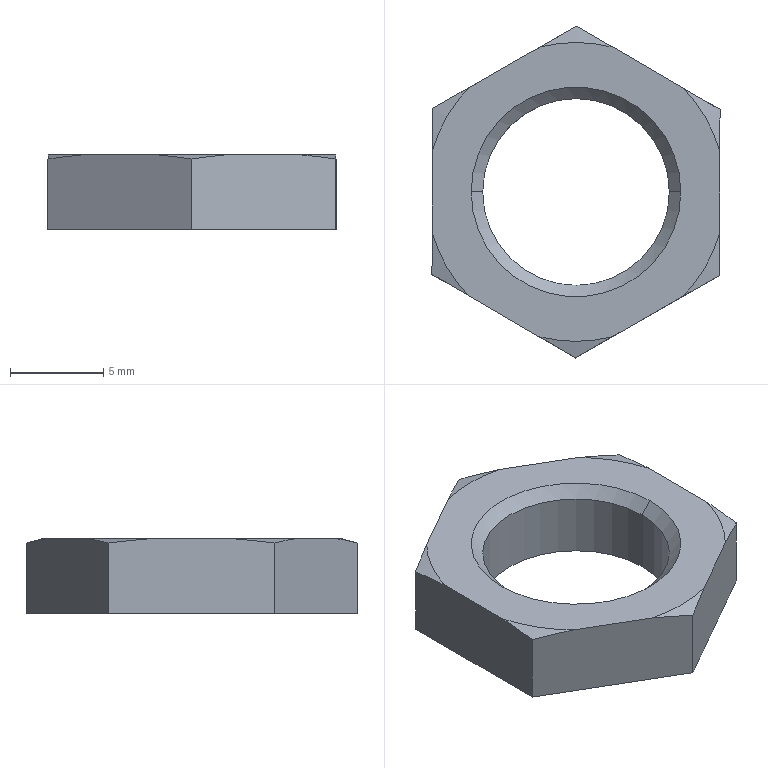Part | SolidWorks | features Cut 3, Chamfer 1, Extrusion 1 | 1 solid | 18 faces | box 15.424 x 17.77 x 4 mm | volume 499.386 mm3 | cone 8 | plane 8 | cylinder 2 | commonest cylinder face diameters 10 x2
STEP:
#1=CARTESIAN_POINT('',(-5.,0.,7.787));
#2=VERTEX_POINT('',#1);
#3=CARTESIAN_POINT('',(5.,0.,7.787));
#4=VERTEX_POINT('',#3);
#5=CARTESIAN_POINT('',(0.,0.,7.787));
#6=DIRECTION('',(0.,0.,1.));
#7=DIRECTION('',(-1.,0.,0.));
#8=AXIS2_PLACEMENT_3D('',#5,#6,#7);
#9=CIRCLE('',#8,5.);
#10=EDGE_CURVE('',#2,#4,#9,.T.);
#11=ORIENTED_EDGE('',*,*,#10,.F.);
#12=CARTESIAN_POINT('',(-5.613,0.,8.4));
#13=VERTEX_POINT('',#12);
#14=CARTESIAN_POINT('',(-5.,0.,7.787));
#15=DIRECTION('',(-0.7071,0.,0.7071));
#16=VECTOR('',#15,1000.);
#17=LINE('',#14,#16);
#18=EDGE_CURVE('',#2,#13,#17,.T.);
#19=ORIENTED_EDGE('',*,*,#18,.T.);
#20=CARTESIAN_POINT('',(5.613,0.,8.4));
#21=VERTEX_POINT('',#20);
#22=CARTESIAN_POINT('',(0.,0.,8.4));
#23=DIRECTION('',(0.,0.,-1.));
#24=DIRECTION('',(-1.,0.,0.));
#25=AXIS2_PLACEMENT_3D('',#22,#23,#24);
#26=CIRCLE('',#25,5.613);
#27=EDGE_CURVE('',#21,#13,#26,.T.);
#28=ORIENTED_EDGE('',*,*,#27,.F.);
#29=CARTESIAN_POINT('',(5.,0.,7.787));
#30=DIRECTION('',(0.7071,0.,0.7071));
#31=VECTOR('',#30,1000.);
#32=LINE('',#29,#31);
#33=EDGE_CURVE('',#4,#21,#32,.T.);
#34=ORIENTED_EDGE('',*,*,#33,.F.);
#35=EDGE_LOOP('',(#11,#19,#28,#34));
#36=FACE_OUTER_BOUND('',#35,.T.);
#37=CARTESIAN_POINT('',(0.,0.,7.787));
#38=DIRECTION('',(0.,0.,1.));
#39=DIRECTION('',(1.,0.,0.));
#40=AXIS2_PLACEMENT_3D('',#37,#38,#39);
#41=CONICAL_SURFACE('',#40,5.,0.7854);
#42=ADVANCED_FACE('',(#36),#41,.F.);
#43=ORIENTED_EDGE('',*,*,#10,.T.);
#44=CARTESIAN_POINT('',(5.,0.,4.4));
#45=VERTEX_POINT('',#44);
#46=CARTESIAN_POINT('',(5.,0.,8.4));
#47=DIRECTION('',(0.,0.,-1.));
#48=VECTOR('',#47,1000.);
#49=LINE('',#46,#48);
#50=EDGE_CURVE('',#4,#45,#49,.T.);
#51=ORIENTED_EDGE('',*,*,#50,.T.);
#52=CARTESIAN_POINT('',(-5.,0.,4.4));
#53=VERTEX_POINT('',#52);
#54=CARTESIAN_POINT('',(0.,0.,4.4));
#55=DIRECTION('',(0.,0.,-1.));
#56=DIRECTION('',(-1.,0.,0.));
#57=AXIS2_PLACEMENT_3D('',#54,#55,#56);
#58=CIRCLE('',#57,5.);
#59=EDGE_CURVE('',#45,#53,#58,.T.);
#60=ORIENTED_EDGE('',*,*,#59,.T.);
#61=CARTESIAN_POINT('',(-5.,0.,8.4));
#62=DIRECTION('',(0.,0.,-1.));
#63=VECTOR('',#62,1000.);
#64=LINE('',#61,#63);
#65=EDGE_CURVE('',#2,#53,#64,.T.);
#66=ORIENTED_EDGE('',*,*,#65,.F.);
#67=EDGE_LOOP('',(#43,#51,#60,#66));
#68=FACE_OUTER_BOUND('',#67,.T.);
#69=CARTESIAN_POINT('',(0.,0.,8.4));
#70=DIRECTION('',(0.,0.,-1.));
#71=DIRECTION('',(-1.,0.,0.));
#72=AXIS2_PLACEMENT_3D('',#69,#70,#71);
#73=CYLINDRICAL_SURFACE('',#72,5.);
#74=ADVANCED_FACE('',(#68),#73,.F.);
#75=CARTESIAN_POINT('',(0.03495,8.885,4.4));
#76=VERTEX_POINT('',#75);
#77=CARTESIAN_POINT('',(7.712,4.412,4.4));
#78=VERTEX_POINT('',#77);
#79=CARTESIAN_POINT('',(7.712,4.412,4.4));
#80=DIRECTION('',(0.8641,-0.5034,0.));
#81=VECTOR('',#80,1000.);
#82=LINE('',#79,#81);
#83=EDGE_CURVE('',#76,#78,#82,.T.);
#84=ORIENTED_EDGE('',*,*,#83,.F.);
#85=CARTESIAN_POINT('',(0.03495,8.885,8.163));
#86=VERTEX_POINT('',#85);
#87=CARTESIAN_POINT('',(0.03495,8.885,8.4));
#88=DIRECTION('',(0.,0.,-1.));
#89=VECTOR('',#88,1000.);
#90=LINE('',#87,#89);
#91=EDGE_CURVE('',#86,#76,#90,.T.);
#92=ORIENTED_EDGE('',*,*,#91,.F.);
#93=CARTESIAN_POINT('',(1.982,7.751,8.4));
#94=VERTEX_POINT('',#93);
#95=CARTESIAN_POINT('',(1.982,7.751,8.4));
#96=CARTESIAN_POINT('',(1.33,8.13,8.345));
#97=CARTESIAN_POINT('',(0.6808,8.509,8.263));
#98=CARTESIAN_POINT('',(0.03495,8.885,8.163));
#99=B_SPLINE_CURVE_WITH_KNOTS('',3,(#95,#96,#97,#98),.UNSPECIFIED.,.F.,.F.,(4,4),(0.01515,0.01738),.UNSPECIFIED.);
#100=EDGE_CURVE('',#94,#86,#99,.T.);
#101=ORIENTED_EDGE('',*,*,#100,.F.);
#102=CARTESIAN_POINT('',(5.765,5.547,8.4));
#103=VERTEX_POINT('',#102);
#104=CARTESIAN_POINT('',(7.712,4.412,8.4));
#105=DIRECTION('',(-0.8641,0.5034,0.));
#106=VECTOR('',#105,1000.);
#107=LINE('',#104,#106);
#108=EDGE_CURVE('',#103,#94,#107,.T.);
#109=ORIENTED_EDGE('',*,*,#108,.F.);
#110=CARTESIAN_POINT('',(7.712,4.412,8.163));
#111=VERTEX_POINT('',#110);
#112=CARTESIAN_POINT('',(7.712,4.412,8.163));
#113=CARTESIAN_POINT('',(7.065,4.789,8.263));
#114=CARTESIAN_POINT('',(6.417,5.167,8.345));
#115=CARTESIAN_POINT('',(5.765,5.547,8.4));
#116=B_SPLINE_CURVE_WITH_KNOTS('',3,(#112,#113,#114,#115),.UNSPECIFIED.,.F.,.F.,(4,4),(0.008541,0.01081),.UNSPECIFIED.);
#117=EDGE_CURVE('',#111,#103,#116,.T.);
#118=ORIENTED_EDGE('',*,*,#117,.F.);
#119=CARTESIAN_POINT('',(7.712,4.412,8.4));
#120=DIRECTION('',(0.,0.,-1.));
#121=VECTOR('',#120,1000.);
#122=LINE('',#119,#121);
#123=EDGE_CURVE('',#111,#78,#122,.T.);
#124=ORIENTED_EDGE('',*,*,#123,.T.);
#125=EDGE_LOOP('',(#84,#92,#101,#109,#118,#124));
#126=FACE_OUTER_BOUND('',#125,.T.);
#127=CARTESIAN_POINT('',(7.712,4.412,8.4));
#128=DIRECTION('',(-0.5034,-0.8641,0.));
#129=DIRECTION('',(0.8641,-0.5034,0.));
#130=AXIS2_PLACEMENT_3D('',#127,#128,#129);
#131=PLANE('',#130);
#132=ADVANCED_FACE('',(#126),#131,.F.);
#133=CARTESIAN_POINT('',(-7.677,4.473,4.4));
#134=VERTEX_POINT('',#133);
#135=CARTESIAN_POINT('',(0.03495,8.885,4.4));
#136=DIRECTION('',(0.868,0.4966,0.));
#137=VECTOR('',#136,1000.);
#138=LINE('',#135,#137);
#139=EDGE_CURVE('',#134,#76,#138,.T.);
#140=ORIENTED_EDGE('',*,*,#139,.F.);
#141=CARTESIAN_POINT('',(-7.677,4.473,8.163));
#142=VERTEX_POINT('',#141);
#143=CARTESIAN_POINT('',(-7.677,4.473,8.4));
#144=DIRECTION('',(0.,0.,-1.));
#145=VECTOR('',#144,1000.);
#146=LINE('',#143,#145);
#147=EDGE_CURVE('',#142,#134,#146,.T.);
#148=ORIENTED_EDGE('',*,*,#147,.F.);
#149=CARTESIAN_POINT('',(-5.721,5.592,8.4));
#150=VERTEX_POINT('',#149);
#151=CARTESIAN_POINT('',(-5.721,5.592,8.4));
#152=CARTESIAN_POINT('',(-6.376,5.217,8.345));
#153=CARTESIAN_POINT('',(-7.028,4.844,8.263));
#154=CARTESIAN_POINT('',(-7.677,4.473,8.163));
#155=B_SPLINE_CURVE_WITH_KNOTS('',3,(#151,#152,#153,#154),.UNSPECIFIED.,.F.,.F.,(4,4),(0.01511,0.01734),.UNSPECIFIED.);
#156=EDGE_CURVE('',#150,#142,#155,.T.);
#157=ORIENTED_EDGE('',*,*,#156,.F.);
#158=CARTESIAN_POINT('',(-1.921,7.766,8.4));
#159=VERTEX_POINT('',#158);
#160=CARTESIAN_POINT('',(0.03495,8.885,8.4));
#161=DIRECTION('',(-0.868,-0.4966,0.));
#162=VECTOR('',#161,1000.);
#163=LINE('',#160,#162);
#164=EDGE_CURVE('',#159,#150,#163,.T.);
#165=ORIENTED_EDGE('',*,*,#164,.F.);
#166=CARTESIAN_POINT('',(0.03495,8.885,8.163));
#167=CARTESIAN_POINT('',(-0.6148,8.513,8.263));
#168=CARTESIAN_POINT('',(-1.266,8.14,8.345));
#169=CARTESIAN_POINT('',(-1.921,7.766,8.4));
#170=B_SPLINE_CURVE_WITH_KNOTS('',3,(#166,#167,#168,#169),.UNSPECIFIED.,.F.,.F.,(4,4),(0.008501,0.01077),.UNSPECIFIED.);
#171=EDGE_CURVE('',#86,#159,#170,.T.);
#172=ORIENTED_EDGE('',*,*,#171,.F.);
#173=ORIENTED_EDGE('',*,*,#91,.T.);
#174=EDGE_LOOP('',(#140,#148,#157,#165,#172,#173));
#175=FACE_OUTER_BOUND('',#174,.T.);
#176=CARTESIAN_POINT('',(0.03495,8.885,8.4));
#177=DIRECTION('',(0.4966,-0.868,0.));
#178=DIRECTION('',(0.868,0.4966,0.));
#179=AXIS2_PLACEMENT_3D('',#176,#177,#178);
#180=PLANE('',#179);
#181=ADVANCED_FACE('',(#175),#180,.F.);
#182=CARTESIAN_POINT('',(-7.712,-4.412,4.4));
#183=VERTEX_POINT('',#182);
#184=CARTESIAN_POINT('',(-7.677,4.473,4.4));
#185=DIRECTION('',(0.003934,1.,0.));
#186=VECTOR('',#185,1000.);
#187=LINE('',#184,#186);
#188=EDGE_CURVE('',#183,#134,#187,.T.);
#189=ORIENTED_EDGE('',*,*,#188,.F.);
#190=CARTESIAN_POINT('',(-7.712,-4.412,8.163));
#191=VERTEX_POINT('',#190);
#192=CARTESIAN_POINT('',(-7.712,-4.412,8.4));
#193=DIRECTION('',(0.,0.,-1.));
#194=VECTOR('',#193,1000.);
#195=LINE('',#192,#194);
#196=EDGE_CURVE('',#191,#183,#195,.T.);
#197=ORIENTED_EDGE('',*,*,#196,.F.);
#198=CARTESIAN_POINT('',(-7.703,-2.159,8.4));
#199=VERTEX_POINT('',#198);
#200=CARTESIAN_POINT('',(-7.703,-2.159,8.4));
#201=CARTESIAN_POINT('',(-7.706,-2.912,8.345));
#202=CARTESIAN_POINT('',(-7.709,-3.665,8.263));
#203=CARTESIAN_POINT('',(-7.712,-4.412,8.163));
#204=B_SPLINE_CURVE_WITH_KNOTS('',3,(#200,#201,#202,#203),.UNSPECIFIED.,.F.,.F.,(4,4),(0.01399,0.01621),.UNSPECIFIED.);
#205=EDGE_CURVE('',#199,#191,#204,.T.);
#206=ORIENTED_EDGE('',*,*,#205,.F.);
#207=CARTESIAN_POINT('',(-7.686,2.219,8.4));
#208=VERTEX_POINT('',#207);
#209=CARTESIAN_POINT('',(-7.677,4.473,8.4));
#210=DIRECTION('',(-0.003934,-1.,0.));
#211=VECTOR('',#210,1000.);
#212=LINE('',#209,#211);
#213=EDGE_CURVE('',#208,#199,#212,.T.);
#214=ORIENTED_EDGE('',*,*,#213,.F.);
#215=CARTESIAN_POINT('',(-7.677,4.473,8.163));
#216=CARTESIAN_POINT('',(-7.68,3.724,8.263));
#217=CARTESIAN_POINT('',(-7.683,2.973,8.345));
#218=CARTESIAN_POINT('',(-7.686,2.219,8.4));
#219=B_SPLINE_CURVE_WITH_KNOTS('',3,(#215,#216,#217,#218),.UNSPECIFIED.,.F.,.F.,(4,4),(0.007369,0.009635),.UNSPECIFIED.);
#220=EDGE_CURVE('',#142,#208,#219,.T.);
#221=ORIENTED_EDGE('',*,*,#220,.F.);
#222=ORIENTED_EDGE('',*,*,#147,.T.);
#223=EDGE_LOOP('',(#189,#197,#206,#214,#221,#222));
#224=FACE_OUTER_BOUND('',#223,.T.);
#225=CARTESIAN_POINT('',(-7.677,4.473,8.4));
#226=DIRECTION('',(1.,-0.003934,0.));
#227=DIRECTION('',(0.003934,1.,0.));
#228=AXIS2_PLACEMENT_3D('',#225,#226,#227);
#229=PLANE('',#228);
#230=ADVANCED_FACE('',(#224),#229,.F.);
#231=CARTESIAN_POINT('',(-0.03495,-8.885,4.4));
#232=VERTEX_POINT('',#231);
#233=CARTESIAN_POINT('',(-7.712,-4.412,4.4));
#234=DIRECTION('',(-0.8641,0.5034,0.));
#235=VECTOR('',#234,1000.);
#236=LINE('',#233,#235);
#237=EDGE_CURVE('',#232,#183,#236,.T.);
#238=ORIENTED_EDGE('',*,*,#237,.F.);
#239=CARTESIAN_POINT('',(-0.03495,-8.885,8.163));
#240=VERTEX_POINT('',#239);
#241=CARTESIAN_POINT('',(-0.03495,-8.885,8.4));
#242=DIRECTION('',(0.,0.,-1.));
#243=VECTOR('',#242,1000.);
#244=LINE('',#241,#243);
#245=EDGE_CURVE('',#240,#232,#244,.T.);
#246=ORIENTED_EDGE('',*,*,#245,.F.);
#247=CARTESIAN_POINT('',(-1.982,-7.751,8.4));
#248=VERTEX_POINT('',#247);
#249=CARTESIAN_POINT('',(-1.982,-7.751,8.4));
#250=CARTESIAN_POINT('',(-1.33,-8.13,8.345));
#251=CARTESIAN_POINT('',(-0.6808,-8.509,8.263));
#252=CARTESIAN_POINT('',(-0.03495,-8.885,8.163));
#253=B_SPLINE_CURVE_WITH_KNOTS('',3,(#249,#250,#251,#252),.UNSPECIFIED.,.F.,.F.,(4,4),(0.01515,0.01738),.UNSPECIFIED.);
#254=EDGE_CURVE('',#248,#240,#253,.T.);
#255=ORIENTED_EDGE('',*,*,#254,.F.);
#256=CARTESIAN_POINT('',(-5.765,-5.547,8.4));
#257=VERTEX_POINT('',#256);
#258=CARTESIAN_POINT('',(-7.712,-4.412,8.4));
#259=DIRECTION('',(0.8641,-0.5034,0.));
#260=VECTOR('',#259,1000.);
#261=LINE('',#258,#260);
#262=EDGE_CURVE('',#257,#248,#261,.T.);
#263=ORIENTED_EDGE('',*,*,#262,.F.);
#264=CARTESIAN_POINT('',(-7.712,-4.412,8.163));
#265=CARTESIAN_POINT('',(-7.065,-4.789,8.263));
#266=CARTESIAN_POINT('',(-6.417,-5.167,8.345));
#267=CARTESIAN_POINT('',(-5.765,-5.547,8.4));
#268=B_SPLINE_CURVE_WITH_KNOTS('',3,(#264,#265,#266,#267),.UNSPECIFIED.,.F.,.F.,(4,4),(0.008541,0.01081),.UNSPECIFIED.);
#269=EDGE_CURVE('',#191,#257,#268,.T.);
#270=ORIENTED_EDGE('',*,*,#269,.F.);
#271=ORIENTED_EDGE('',*,*,#196,.T.);
#272=EDGE_LOOP('',(#238,#246,#255,#263,#270,#271));
#273=FACE_OUTER_BOUND('',#272,.T.);
#274=CARTESIAN_POINT('',(-7.712,-4.412,8.4));
#275=DIRECTION('',(0.5034,0.8641,0.));
#276=DIRECTION('',(-0.8641,0.5034,0.));
#277=AXIS2_PLACEMENT_3D('',#274,#275,#276);
#278=PLANE('',#277);
#279=ADVANCED_FACE('',(#273),#278,.F.);
#280=CARTESIAN_POINT('',(7.677,-4.473,4.4));
#281=VERTEX_POINT('',#280);
#282=CARTESIAN_POINT('',(-0.03495,-8.885,4.4));
#283=DIRECTION('',(-0.868,-0.4966,0.));
#284=VECTOR('',#283,1000.);
#285=LINE('',#282,#284);
#286=EDGE_CURVE('',#281,#232,#285,.T.);
#287=ORIENTED_EDGE('',*,*,#286,.F.);
#288=CARTESIAN_POINT('',(7.677,-4.473,8.163));
#289=VERTEX_POINT('',#288);
#290=CARTESIAN_POINT('',(7.677,-4.473,8.4));
#291=DIRECTION('',(0.,0.,-1.));
#292=VECTOR('',#291,1000.);
#293=LINE('',#290,#292);
#294=EDGE_CURVE('',#289,#281,#293,.T.);
#295=ORIENTED_EDGE('',*,*,#294,.F.);
#296=CARTESIAN_POINT('',(5.721,-5.592,8.4));
#297=VERTEX_POINT('',#296);
#298=CARTESIAN_POINT('',(5.721,-5.592,8.4));
#299=CARTESIAN_POINT('',(6.376,-5.217,8.345));
#300=CARTESIAN_POINT('',(7.028,-4.844,8.263));
#301=CARTESIAN_POINT('',(7.677,-4.473,8.163));
#302=B_SPLINE_CURVE_WITH_KNOTS('',3,(#298,#299,#300,#301),.UNSPECIFIED.,.F.,.F.,(4,4),(0.01511,0.01734),.UNSPECIFIED.);
#303=EDGE_CURVE('',#297,#289,#302,.T.);
#304=ORIENTED_EDGE('',*,*,#303,.F.);
#305=CARTESIAN_POINT('',(1.921,-7.766,8.4));
#306=VERTEX_POINT('',#305);
#307=CARTESIAN_POINT('',(-0.03495,-8.885,8.4));
#308=DIRECTION('',(0.868,0.4966,0.));
#309=VECTOR('',#308,1000.);
#310=LINE('',#307,#309);
#311=EDGE_CURVE('',#306,#297,#310,.T.);
#312=ORIENTED_EDGE('',*,*,#311,.F.);
#313=CARTESIAN_POINT('',(-0.03495,-8.885,8.163));
#314=CARTESIAN_POINT('',(0.6148,-8.513,8.263));
#315=CARTESIAN_POINT('',(1.266,-8.14,8.345));
#316=CARTESIAN_POINT('',(1.921,-7.766,8.4));
#317=B_SPLINE_CURVE_WITH_KNOTS('',3,(#313,#314,#315,#316),.UNSPECIFIED.,.F.,.F.,(4,4),(0.008501,0.01077),.UNSPECIFIED.);
#318=EDGE_CURVE('',#240,#306,#317,.T.);
#319=ORIENTED_EDGE('',*,*,#318,.F.);
#320=ORIENTED_EDGE('',*,*,#245,.T.);
#321=EDGE_LOOP('',(#287,#295,#304,#312,#319,#320));
#322=FACE_OUTER_BOUND('',#321,.T.);
#323=CARTESIAN_POINT('',(-0.03495,-8.885,8.4));
#324=DIRECTION('',(-0.4966,0.868,0.));
#325=DIRECTION('',(-0.868,-0.4966,0.));
#326=AXIS2_PLACEMENT_3D('',#323,#324,#325);
#327=PLANE('',#326);
#328=ADVANCED_FACE('',(#322),#327,.F.);
#329=CARTESIAN_POINT('',(7.677,-4.473,4.4));
#330=DIRECTION('',(-0.003934,-1.,0.));
#331=VECTOR('',#330,1000.);
#332=LINE('',#329,#331);
#333=EDGE_CURVE('',#78,#281,#332,.T.);
#334=ORIENTED_EDGE('',*,*,#333,.F.);
#335=ORIENTED_EDGE('',*,*,#123,.F.);
#336=CARTESIAN_POINT('',(7.703,2.159,8.4));
#337=VERTEX_POINT('',#336);
#338=CARTESIAN_POINT('',(7.703,2.159,8.4));
#339=CARTESIAN_POINT('',(7.706,2.912,8.345));
#340=CARTESIAN_POINT('',(7.709,3.665,8.263));
#341=CARTESIAN_POINT('',(7.712,4.412,8.163));
#342=B_SPLINE_CURVE_WITH_KNOTS('',3,(#338,#339,#340,#341),.UNSPECIFIED.,.F.,.F.,(4,4),(0.01399,0.01621),.UNSPECIFIED.);
#343=EDGE_CURVE('',#337,#111,#342,.T.);
#344=ORIENTED_EDGE('',*,*,#343,.F.);
#345=CARTESIAN_POINT('',(7.686,-2.219,8.4));
#346=VERTEX_POINT('',#345);
#347=CARTESIAN_POINT('',(7.677,-4.473,8.4));
#348=DIRECTION('',(0.003934,1.,0.));
#349=VECTOR('',#348,1000.);
#350=LINE('',#347,#349);
#351=EDGE_CURVE('',#346,#337,#350,.T.);
#352=ORIENTED_EDGE('',*,*,#351,.F.);
#353=CARTESIAN_POINT('',(7.677,-4.473,8.163));
#354=CARTESIAN_POINT('',(7.68,-3.724,8.263));
#355=CARTESIAN_POINT('',(7.683,-2.973,8.345));
#356=CARTESIAN_POINT('',(7.686,-2.219,8.4));
#357=B_SPLINE_CURVE_WITH_KNOTS('',3,(#353,#354,#355,#356),.UNSPECIFIED.,.F.,.F.,(4,4),(0.007369,0.009635),.UNSPECIFIED.);
#358=EDGE_CURVE('',#289,#346,#357,.T.);
#359=ORIENTED_EDGE('',*,*,#358,.F.);
#360=ORIENTED_EDGE('',*,*,#294,.T.);
#361=EDGE_LOOP('',(#334,#335,#344,#352,#359,#360));
#362=FACE_OUTER_BOUND('',#361,.T.);
#363=CARTESIAN_POINT('',(7.677,-4.473,8.4));
#364=DIRECTION('',(-1.,0.003934,0.));
#365=DIRECTION('',(-0.003934,-1.,0.));
#366=AXIS2_PLACEMENT_3D('',#363,#364,#365);
#367=PLANE('',#366);
#368=ADVANCED_FACE('',(#362),#367,.F.);
#369=ORIENTED_EDGE('',*,*,#50,.F.);
#370=CARTESIAN_POINT('',(0.,0.,7.787));
#371=DIRECTION('',(0.,0.,1.));
#372=DIRECTION('',(-1.,0.,0.));
#373=AXIS2_PLACEMENT_3D('',#370,#371,#372);
#374=CIRCLE('',#373,5.);
#375=EDGE_CURVE('',#4,#2,#374,.T.);
#376=ORIENTED_EDGE('',*,*,#375,.T.);
#377=ORIENTED_EDGE('',*,*,#65,.T.);
#378=CARTESIAN_POINT('',(0.,0.,4.4));
#379=DIRECTION('',(0.,0.,-1.));
#380=DIRECTION('',(-1.,0.,0.));
#381=AXIS2_PLACEMENT_3D('',#378,#379,#380);
#382=CIRCLE('',#381,5.);
#383=EDGE_CURVE('',#53,#45,#382,.T.);
#384=ORIENTED_EDGE('',*,*,#383,.T.);
#385=EDGE_LOOP('',(#369,#376,#377,#384));
#386=FACE_OUTER_BOUND('',#385,.T.);
#387=CARTESIAN_POINT('',(0.,0.,8.4));
#388=DIRECTION('',(0.,0.,-1.));
#389=DIRECTION('',(-1.,0.,0.));
#390=AXIS2_PLACEMENT_3D('',#387,#388,#389);
#391=CYLINDRICAL_SURFACE('',#390,5.);
#392=ADVANCED_FACE('',(#386),#391,.F.);
#393=ORIENTED_EDGE('',*,*,#27,.T.);
#394=CARTESIAN_POINT('',(0.,0.,8.4));
#395=DIRECTION('',(0.,0.,-1.));
#396=DIRECTION('',(-1.,0.,0.));
#397=AXIS2_PLACEMENT_3D('',#394,#395,#396);
#398=CIRCLE('',#397,5.613);
#399=EDGE_CURVE('',#13,#21,#398,.T.);
#400=ORIENTED_EDGE('',*,*,#399,.T.);
#401=EDGE_LOOP('',(#393,#400));
#402=FACE_BOUND('',#401,.T.);
#403=CARTESIAN_POINT('',(0.,0.,8.4));
#404=DIRECTION('',(0.,0.,-1.));
#405=DIRECTION('',(-1.,0.,0.));
#406=AXIS2_PLACEMENT_3D('',#403,#404,#405);
#407=CIRCLE('',#406,8.);
#408=EDGE_CURVE('',#208,#150,#407,.T.);
#409=ORIENTED_EDGE('',*,*,#408,.F.);
#410=ORIENTED_EDGE('',*,*,#213,.T.);
#411=CARTESIAN_POINT('',(0.,0.,8.4));
#412=DIRECTION('',(0.,0.,-1.));
#413=DIRECTION('',(-1.,0.,0.));
#414=AXIS2_PLACEMENT_3D('',#411,#412,#413);
#415=CIRCLE('',#414,8.);
#416=EDGE_CURVE('',#257,#199,#415,.T.);
#417=ORIENTED_EDGE('',*,*,#416,.F.);
#418=ORIENTED_EDGE('',*,*,#262,.T.);
#419=CARTESIAN_POINT('',(0.,0.,8.4));
#420=DIRECTION('',(0.,0.,-1.));
#421=DIRECTION('',(-1.,0.,0.));
#422=AXIS2_PLACEMENT_3D('',#419,#420,#421);
#423=CIRCLE('',#422,8.);
#424=EDGE_CURVE('',#306,#248,#423,.T.);
#425=ORIENTED_EDGE('',*,*,#424,.F.);
#426=ORIENTED_EDGE('',*,*,#311,.T.);
#427=CARTESIAN_POINT('',(0.,0.,8.4));
#428=DIRECTION('',(0.,0.,-1.));
#429=DIRECTION('',(-1.,0.,0.));
#430=AXIS2_PLACEMENT_3D('',#427,#428,#429);
#431=CIRCLE('',#430,8.);
#432=EDGE_CURVE('',#346,#297,#431,.T.);
#433=ORIENTED_EDGE('',*,*,#432,.F.);
#434=ORIENTED_EDGE('',*,*,#351,.T.);
#435=CARTESIAN_POINT('',(0.,0.,8.4));
#436=DIRECTION('',(0.,0.,1.));
#437=DIRECTION('',(1.,0.,0.));
#438=AXIS2_PLACEMENT_3D('',#435,#436,#437);
#439=CIRCLE('',#438,8.);
#440=EDGE_CURVE('',#337,#103,#439,.T.);
#441=ORIENTED_EDGE('',*,*,#440,.T.);
#442=ORIENTED_EDGE('',*,*,#108,.T.);
#443=CARTESIAN_POINT('',(0.,0.,8.4));
#444=DIRECTION('',(0.,0.,-1.));
#445=DIRECTION('',(-1.,0.,0.));
#446=AXIS2_PLACEMENT_3D('',#443,#444,#445);
#447=CIRCLE('',#446,8.);
#448=EDGE_CURVE('',#159,#94,#447,.T.);
#449=ORIENTED_EDGE('',*,*,#448,.F.);
#450=ORIENTED_EDGE('',*,*,#164,.T.);
#451=EDGE_LOOP('',(#409,#410,#417,#418,#425,#426,#433,#434,#441,#442,#449,#450));
#452=FACE_OUTER_BOUND('',#451,.T.);
#453=CARTESIAN_POINT('',(7.712,4.412,8.4));
#454=DIRECTION('',(0.,0.,-1.));
#455=DIRECTION('',(-1.,0.,0.));
#456=AXIS2_PLACEMENT_3D('',#453,#454,#455);
#457=PLANE('',#456);
#458=ADVANCED_FACE('',(#402,#452),#457,.F.);
#459=ORIENTED_EDGE('',*,*,#205,.T.);
#460=ORIENTED_EDGE('',*,*,#269,.T.);
#461=ORIENTED_EDGE('',*,*,#416,.T.);
#462=EDGE_LOOP('',(#459,#460,#461));
#463=FACE_OUTER_BOUND('',#462,.T.);
#464=CARTESIAN_POINT('',(0.,0.,8.4));
#465=DIRECTION('',(0.,0.,-1.));
#466=DIRECTION('',(1.,0.,0.));
#467=AXIS2_PLACEMENT_3D('',#464,#465,#466);
#468=CONICAL_SURFACE('',#467,8.,1.309);
#469=ADVANCED_FACE('',(#463),#468,.T.);
#470=ORIENTED_EDGE('',*,*,#254,.T.);
#471=ORIENTED_EDGE('',*,*,#318,.T.);
#472=ORIENTED_EDGE('',*,*,#424,.T.);
#473=EDGE_LOOP('',(#470,#471,#472));
#474=FACE_OUTER_BOUND('',#473,.T.);
#475=CARTESIAN_POINT('',(0.,0.,8.4));
#476=DIRECTION('',(0.,0.,-1.));
#477=DIRECTION('',(1.,0.,0.));
#478=AXIS2_PLACEMENT_3D('',#475,#476,#477);
#479=CONICAL_SURFACE('',#478,8.,1.309);
#480=ADVANCED_FACE('',(#474),#479,.T.);
#481=ORIENTED_EDGE('',*,*,#303,.T.);
#482=ORIENTED_EDGE('',*,*,#358,.T.);
#483=ORIENTED_EDGE('',*,*,#432,.T.);
#484=EDGE_LOOP('',(#481,#482,#483));
#485=FACE_OUTER_BOUND('',#484,.T.);
#486=CARTESIAN_POINT('',(0.,0.,8.4));
#487=DIRECTION('',(0.,0.,-1.));
#488=DIRECTION('',(1.,0.,0.));
#489=AXIS2_PLACEMENT_3D('',#486,#487,#488);
#490=CONICAL_SURFACE('',#489,8.,1.309);
#491=ADVANCED_FACE('',(#485),#490,.T.);
#492=ORIENTED_EDGE('',*,*,#117,.T.);
#493=ORIENTED_EDGE('',*,*,#440,.F.);
#494=ORIENTED_EDGE('',*,*,#343,.T.);
#495=EDGE_LOOP('',(#492,#493,#494));
#496=FACE_OUTER_BOUND('',#495,.T.);
#497=CARTESIAN_POINT('',(0.,0.,8.4));
#498=DIRECTION('',(0.,0.,-1.));
#499=DIRECTION('',(1.,0.,0.));
#500=AXIS2_PLACEMENT_3D('',#497,#498,#499);
#501=CONICAL_SURFACE('',#500,8.,1.309);
#502=ADVANCED_FACE('',(#496),#501,.T.);
#503=ORIENTED_EDGE('',*,*,#100,.T.);
#504=ORIENTED_EDGE('',*,*,#171,.T.);
#505=ORIENTED_EDGE('',*,*,#448,.T.);
#506=EDGE_LOOP('',(#503,#504,#505));
#507=FACE_OUTER_BOUND('',#506,.T.);
#508=CARTESIAN_POINT('',(0.,0.,8.4));
#509=DIRECTION('',(0.,0.,-1.));
#510=DIRECTION('',(1.,0.,0.));
#511=AXIS2_PLACEMENT_3D('',#508,#509,#510);
#512=CONICAL_SURFACE('',#511,8.,1.309);
#513=ADVANCED_FACE('',(#507),#512,.T.);
#514=ORIENTED_EDGE('',*,*,#156,.T.);
#515=ORIENTED_EDGE('',*,*,#220,.T.);
#516=ORIENTED_EDGE('',*,*,#408,.T.);
#517=EDGE_LOOP('',(#514,#515,#516));
#518=FACE_OUTER_BOUND('',#517,.T.);
#519=CARTESIAN_POINT('',(0.,0.,8.4));
#520=DIRECTION('',(0.,0.,-1.));
#521=DIRECTION('',(1.,0.,0.));
#522=AXIS2_PLACEMENT_3D('',#519,#520,#521);
#523=CONICAL_SURFACE('',#522,8.,1.309);
#524=ADVANCED_FACE('',(#518),#523,.T.);
#525=ORIENTED_EDGE('',*,*,#18,.F.);
#526=ORIENTED_EDGE('',*,*,#375,.F.);
#527=ORIENTED_EDGE('',*,*,#33,.T.);
#528=ORIENTED_EDGE('',*,*,#399,.F.);
#529=EDGE_LOOP('',(#525,#526,#527,#528));
#530=FACE_OUTER_BOUND('',#529,.T.);
#531=CARTESIAN_POINT('',(0.,0.,7.787));
#532=DIRECTION('',(0.,0.,1.));
#533=DIRECTION('',(1.,0.,0.));
#534=AXIS2_PLACEMENT_3D('',#531,#532,#533);
#535=CONICAL_SURFACE('',#534,5.,0.7854);
#536=ADVANCED_FACE('',(#530),#535,.F.);
#537=ORIENTED_EDGE('',*,*,#383,.F.);
#538=ORIENTED_EDGE('',*,*,#59,.F.);
#539=EDGE_LOOP('',(#537,#538));
#540=FACE_BOUND('',#539,.T.);
#541=ORIENTED_EDGE('',*,*,#83,.T.);
#542=ORIENTED_EDGE('',*,*,#333,.T.);
#543=ORIENTED_EDGE('',*,*,#286,.T.);
#544=ORIENTED_EDGE('',*,*,#237,.T.);
#545=ORIENTED_EDGE('',*,*,#188,.T.);
#546=ORIENTED_EDGE('',*,*,#139,.T.);
#547=EDGE_LOOP('',(#541,#542,#543,#544,#545,#546));
#548=FACE_OUTER_BOUND('',#547,.T.);
#549=CARTESIAN_POINT('',(0.,0.,4.4));
#550=DIRECTION('',(0.,0.,-1.));
#551=DIRECTION('',(-1.,0.,0.));
#552=AXIS2_PLACEMENT_3D('',#549,#550,#551);
#553=PLANE('',#552);
#554=ADVANCED_FACE('',(#540,#548),#553,.T.);
#555=CLOSED_SHELL('',(#42,#74,#132,#181,#230,#279,#328,#368,#392,#458,#469,#480,#491,#502,#513,#524,#536,#554));
#556=MANIFOLD_SOLID_BREP('',#555);
#557=CARTESIAN_POINT('',(0.,0.,0.));
#558=DIRECTION('',(0.,0.,1.));
#559=DIRECTION('',(1.,0.,0.));
#560=AXIS2_PLACEMENT_3D('',#557,#558,#559);
#561=(LENGTH_UNIT()NAMED_UNIT(*)SI_UNIT(.MILLI.,.METRE.));
#562=UNCERTAINTY_MEASURE_WITH_UNIT(LENGTH_MEASURE(0.00001),#561,'','');
#563=(NAMED_UNIT(*)PLANE_ANGLE_UNIT()SI_UNIT($,.RADIAN.));
#564=(NAMED_UNIT(*)SI_UNIT($,.STERADIAN.)SOLID_ANGLE_UNIT());
#565=(GEOMETRIC_REPRESENTATION_CONTEXT(3)GLOBAL_UNCERTAINTY_ASSIGNED_CONTEXT((#562))GLOBAL_UNIT_ASSIGNED_CONTEXT((#561,#563,#564))REPRESENTATION_CONTEXT('',''));
#566=ADVANCED_BREP_SHAPE_REPRESENTATION('',(#556,#560),#565);